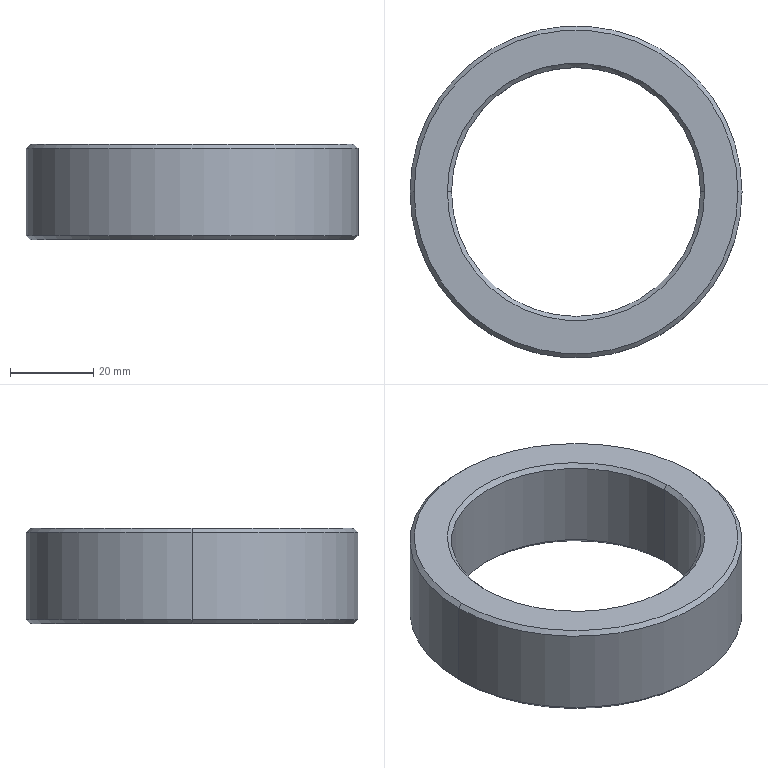Part | SolidWorks | features Chamfer 1, Extrusion 1 | 1 solid | 14 faces | box 80 x 80 x 23 mm | volume 50140 mm3 | cone 8 | cylinder 4 | plane 2 | commonest cylinder face diameters 60 x2 80 x2
STEP:
#1=CARTESIAN_POINT('',(39.,0.,11.5));
#2=VERTEX_POINT('',#1);
#3=CARTESIAN_POINT('',(-39.,0.,11.5));
#4=VERTEX_POINT('',#3);
#5=CARTESIAN_POINT('',(0.,0.,11.5));
#6=DIRECTION('',(0.,0.,1.));
#7=DIRECTION('',(1.,0.,0.));
#8=AXIS2_PLACEMENT_3D('',#5,#6,#7);
#9=CIRCLE('',#8,39.);
#10=EDGE_CURVE('',#2,#4,#9,.T.);
#11=ORIENTED_EDGE('',*,*,#10,.F.);
#12=CARTESIAN_POINT('',(40.,0.,10.5));
#13=VERTEX_POINT('',#12);
#14=CARTESIAN_POINT('',(39.,0.,11.5));
#15=DIRECTION('',(0.7071,0.,-0.7071));
#16=VECTOR('',#15,1000.);
#17=LINE('',#14,#16);
#18=EDGE_CURVE('',#2,#13,#17,.T.);
#19=ORIENTED_EDGE('',*,*,#18,.T.);
#20=CARTESIAN_POINT('',(-40.,0.,10.5));
#21=VERTEX_POINT('',#20);
#22=CARTESIAN_POINT('',(0.,0.,10.5));
#23=DIRECTION('',(0.,0.,-1.));
#24=DIRECTION('',(1.,0.,0.));
#25=AXIS2_PLACEMENT_3D('',#22,#23,#24);
#26=CIRCLE('',#25,40.);
#27=EDGE_CURVE('',#21,#13,#26,.T.);
#28=ORIENTED_EDGE('',*,*,#27,.F.);
#29=CARTESIAN_POINT('',(-39.,0.,11.5));
#30=DIRECTION('',(-0.7071,0.,-0.7071));
#31=VECTOR('',#30,1000.);
#32=LINE('',#29,#31);
#33=EDGE_CURVE('',#4,#21,#32,.T.);
#34=ORIENTED_EDGE('',*,*,#33,.F.);
#35=EDGE_LOOP('',(#11,#19,#28,#34));
#36=FACE_OUTER_BOUND('',#35,.T.);
#37=CARTESIAN_POINT('',(0.,0.,11.5));
#38=DIRECTION('',(0.,0.,-1.));
#39=DIRECTION('',(-1.,0.,0.));
#40=AXIS2_PLACEMENT_3D('',#37,#38,#39);
#41=CONICAL_SURFACE('',#40,39.,0.7854);
#42=ADVANCED_FACE('',(#36),#41,.T.);
#43=CARTESIAN_POINT('',(-30.,0.,10.5));
#44=VERTEX_POINT('',#43);
#45=CARTESIAN_POINT('',(30.,0.,10.5));
#46=VERTEX_POINT('',#45);
#47=CARTESIAN_POINT('',(0.,0.,10.5));
#48=DIRECTION('',(0.,0.,1.));
#49=DIRECTION('',(1.,0.,0.));
#50=AXIS2_PLACEMENT_3D('',#47,#48,#49);
#51=CIRCLE('',#50,30.);
#52=EDGE_CURVE('',#44,#46,#51,.T.);
#53=ORIENTED_EDGE('',*,*,#52,.F.);
#54=CARTESIAN_POINT('',(-31.,0.,11.5));
#55=VERTEX_POINT('',#54);
#56=CARTESIAN_POINT('',(-30.,0.,10.5));
#57=DIRECTION('',(-0.7071,0.,0.7071));
#58=VECTOR('',#57,1000.);
#59=LINE('',#56,#58);
#60=EDGE_CURVE('',#44,#55,#59,.T.);
#61=ORIENTED_EDGE('',*,*,#60,.T.);
#62=CARTESIAN_POINT('',(31.,0.,11.5));
#63=VERTEX_POINT('',#62);
#64=CARTESIAN_POINT('',(0.,0.,11.5));
#65=DIRECTION('',(0.,0.,-1.));
#66=DIRECTION('',(1.,0.,0.));
#67=AXIS2_PLACEMENT_3D('',#64,#65,#66);
#68=CIRCLE('',#67,31.);
#69=EDGE_CURVE('',#63,#55,#68,.T.);
#70=ORIENTED_EDGE('',*,*,#69,.F.);
#71=CARTESIAN_POINT('',(30.,0.,10.5));
#72=DIRECTION('',(0.7071,0.,0.7071));
#73=VECTOR('',#72,1000.);
#74=LINE('',#71,#73);
#75=EDGE_CURVE('',#46,#63,#74,.T.);
#76=ORIENTED_EDGE('',*,*,#75,.F.);
#77=EDGE_LOOP('',(#53,#61,#70,#76));
#78=FACE_OUTER_BOUND('',#77,.T.);
#79=CARTESIAN_POINT('',(0.,0.,10.5));
#80=DIRECTION('',(0.,0.,1.));
#81=DIRECTION('',(1.,0.,0.));
#82=AXIS2_PLACEMENT_3D('',#79,#80,#81);
#83=CONICAL_SURFACE('',#82,30.,0.7854);
#84=ADVANCED_FACE('',(#78),#83,.F.);
#85=CARTESIAN_POINT('',(-39.,0.,-11.5));
#86=VERTEX_POINT('',#85);
#87=CARTESIAN_POINT('',(39.,0.,-11.5));
#88=VERTEX_POINT('',#87);
#89=CARTESIAN_POINT('',(0.,0.,-11.5));
#90=DIRECTION('',(0.,0.,-1.));
#91=DIRECTION('',(1.,0.,0.));
#92=AXIS2_PLACEMENT_3D('',#89,#90,#91);
#93=CIRCLE('',#92,39.);
#94=EDGE_CURVE('',#86,#88,#93,.T.);
#95=ORIENTED_EDGE('',*,*,#94,.F.);
#96=CARTESIAN_POINT('',(-40.,0.,-10.5));
#97=VERTEX_POINT('',#96);
#98=CARTESIAN_POINT('',(-40.,0.,-10.5));
#99=DIRECTION('',(-0.7071,0.,0.7071));
#100=VECTOR('',#99,1000.);
#101=LINE('',#98,#100);
#102=EDGE_CURVE('',#86,#97,#101,.T.);
#103=ORIENTED_EDGE('',*,*,#102,.T.);
#104=CARTESIAN_POINT('',(40.,0.,-10.5));
#105=VERTEX_POINT('',#104);
#106=CARTESIAN_POINT('',(0.,0.,-10.5));
#107=DIRECTION('',(0.,0.,1.));
#108=DIRECTION('',(1.,0.,0.));
#109=AXIS2_PLACEMENT_3D('',#106,#107,#108);
#110=CIRCLE('',#109,40.);
#111=EDGE_CURVE('',#105,#97,#110,.T.);
#112=ORIENTED_EDGE('',*,*,#111,.F.);
#113=CARTESIAN_POINT('',(40.,0.,-10.5));
#114=DIRECTION('',(0.7071,0.,0.7071));
#115=VECTOR('',#114,1000.);
#116=LINE('',#113,#115);
#117=EDGE_CURVE('',#88,#105,#116,.T.);
#118=ORIENTED_EDGE('',*,*,#117,.F.);
#119=EDGE_LOOP('',(#95,#103,#112,#118));
#120=FACE_OUTER_BOUND('',#119,.T.);
#121=CARTESIAN_POINT('',(0.,0.,-10.5));
#122=DIRECTION('',(0.,0.,1.));
#123=DIRECTION('',(1.,0.,0.));
#124=AXIS2_PLACEMENT_3D('',#121,#122,#123);
#125=CONICAL_SURFACE('',#124,40.,0.7854);
#126=ADVANCED_FACE('',(#120),#125,.T.);
#127=CARTESIAN_POINT('',(30.,0.,-10.5));
#128=VERTEX_POINT('',#127);
#129=CARTESIAN_POINT('',(-30.,0.,-10.5));
#130=VERTEX_POINT('',#129);
#131=CARTESIAN_POINT('',(0.,0.,-10.5));
#132=DIRECTION('',(0.,0.,-1.));
#133=DIRECTION('',(1.,0.,0.));
#134=AXIS2_PLACEMENT_3D('',#131,#132,#133);
#135=CIRCLE('',#134,30.);
#136=EDGE_CURVE('',#128,#130,#135,.T.);
#137=ORIENTED_EDGE('',*,*,#136,.F.);
#138=CARTESIAN_POINT('',(31.,0.,-11.5));
#139=VERTEX_POINT('',#138);
#140=CARTESIAN_POINT('',(31.,0.,-11.5));
#141=DIRECTION('',(0.7071,0.,-0.7071));
#142=VECTOR('',#141,1000.);
#143=LINE('',#140,#142);
#144=EDGE_CURVE('',#128,#139,#143,.T.);
#145=ORIENTED_EDGE('',*,*,#144,.T.);
#146=CARTESIAN_POINT('',(-31.,0.,-11.5));
#147=VERTEX_POINT('',#146);
#148=CARTESIAN_POINT('',(0.,0.,-11.5));
#149=DIRECTION('',(0.,0.,1.));
#150=DIRECTION('',(1.,0.,0.));
#151=AXIS2_PLACEMENT_3D('',#148,#149,#150);
#152=CIRCLE('',#151,31.);
#153=EDGE_CURVE('',#147,#139,#152,.T.);
#154=ORIENTED_EDGE('',*,*,#153,.F.);
#155=CARTESIAN_POINT('',(-31.,0.,-11.5));
#156=DIRECTION('',(-0.7071,0.,-0.7071));
#157=VECTOR('',#156,1000.);
#158=LINE('',#155,#157);
#159=EDGE_CURVE('',#130,#147,#158,.T.);
#160=ORIENTED_EDGE('',*,*,#159,.F.);
#161=EDGE_LOOP('',(#137,#145,#154,#160));
#162=FACE_OUTER_BOUND('',#161,.T.);
#163=CARTESIAN_POINT('',(0.,0.,-11.5));
#164=DIRECTION('',(0.,0.,-1.));
#165=DIRECTION('',(-1.,0.,0.));
#166=AXIS2_PLACEMENT_3D('',#163,#164,#165);
#167=CONICAL_SURFACE('',#166,31.,0.7854);
#168=ADVANCED_FACE('',(#162),#167,.F.);
#169=ORIENTED_EDGE('',*,*,#52,.T.);
#170=CARTESIAN_POINT('',(30.,0.,11.5));
#171=DIRECTION('',(0.,0.,-1.));
#172=VECTOR('',#171,1000.);
#173=LINE('',#170,#172);
#174=EDGE_CURVE('',#46,#128,#173,.T.);
#175=ORIENTED_EDGE('',*,*,#174,.T.);
#176=ORIENTED_EDGE('',*,*,#136,.T.);
#177=CARTESIAN_POINT('',(-30.,0.,11.5));
#178=DIRECTION('',(0.,0.,-1.));
#179=VECTOR('',#178,1000.);
#180=LINE('',#177,#179);
#181=EDGE_CURVE('',#44,#130,#180,.T.);
#182=ORIENTED_EDGE('',*,*,#181,.F.);
#183=EDGE_LOOP('',(#169,#175,#176,#182));
#184=FACE_OUTER_BOUND('',#183,.T.);
#185=CARTESIAN_POINT('',(0.,0.,11.5));
#186=DIRECTION('',(0.,0.,-1.));
#187=DIRECTION('',(-1.,0.,0.));
#188=AXIS2_PLACEMENT_3D('',#185,#186,#187);
#189=CYLINDRICAL_SURFACE('',#188,30.);
#190=ADVANCED_FACE('',(#184),#189,.F.);
#191=ORIENTED_EDGE('',*,*,#27,.T.);
#192=CARTESIAN_POINT('',(40.,0.,11.5));
#193=DIRECTION('',(0.,0.,-1.));
#194=VECTOR('',#193,1000.);
#195=LINE('',#192,#194);
#196=EDGE_CURVE('',#13,#105,#195,.T.);
#197=ORIENTED_EDGE('',*,*,#196,.T.);
#198=ORIENTED_EDGE('',*,*,#111,.T.);
#199=CARTESIAN_POINT('',(-40.,0.,11.5));
#200=DIRECTION('',(0.,0.,-1.));
#201=VECTOR('',#200,1000.);
#202=LINE('',#199,#201);
#203=EDGE_CURVE('',#21,#97,#202,.T.);
#204=ORIENTED_EDGE('',*,*,#203,.F.);
#205=EDGE_LOOP('',(#191,#197,#198,#204));
#206=FACE_OUTER_BOUND('',#205,.T.);
#207=CARTESIAN_POINT('',(0.,0.,11.5));
#208=DIRECTION('',(0.,0.,-1.));
#209=DIRECTION('',(-1.,0.,0.));
#210=AXIS2_PLACEMENT_3D('',#207,#208,#209);
#211=CYLINDRICAL_SURFACE('',#210,40.);
#212=ADVANCED_FACE('',(#206),#211,.T.);
#213=ORIENTED_EDGE('',*,*,#69,.T.);
#214=CARTESIAN_POINT('',(0.,0.,11.5));
#215=DIRECTION('',(0.,0.,-1.));
#216=DIRECTION('',(1.,0.,0.));
#217=AXIS2_PLACEMENT_3D('',#214,#215,#216);
#218=CIRCLE('',#217,31.);
#219=EDGE_CURVE('',#55,#63,#218,.T.);
#220=ORIENTED_EDGE('',*,*,#219,.T.);
#221=EDGE_LOOP('',(#213,#220));
#222=FACE_BOUND('',#221,.T.);
#223=CARTESIAN_POINT('',(0.,0.,11.5));
#224=DIRECTION('',(0.,0.,1.));
#225=DIRECTION('',(1.,0.,0.));
#226=AXIS2_PLACEMENT_3D('',#223,#224,#225);
#227=CIRCLE('',#226,39.);
#228=EDGE_CURVE('',#4,#2,#227,.T.);
#229=ORIENTED_EDGE('',*,*,#228,.T.);
#230=ORIENTED_EDGE('',*,*,#10,.T.);
#231=EDGE_LOOP('',(#229,#230));
#232=FACE_OUTER_BOUND('',#231,.T.);
#233=CARTESIAN_POINT('',(0.,0.,11.5));
#234=DIRECTION('',(0.,0.,1.));
#235=DIRECTION('',(1.,0.,0.));
#236=AXIS2_PLACEMENT_3D('',#233,#234,#235);
#237=PLANE('',#236);
#238=ADVANCED_FACE('',(#222,#232),#237,.T.);
#239=ORIENTED_EDGE('',*,*,#153,.T.);
#240=CARTESIAN_POINT('',(0.,0.,-11.5));
#241=DIRECTION('',(0.,0.,1.));
#242=DIRECTION('',(1.,0.,0.));
#243=AXIS2_PLACEMENT_3D('',#240,#241,#242);
#244=CIRCLE('',#243,31.);
#245=EDGE_CURVE('',#139,#147,#244,.T.);
#246=ORIENTED_EDGE('',*,*,#245,.T.);
#247=EDGE_LOOP('',(#239,#246));
#248=FACE_BOUND('',#247,.T.);
#249=CARTESIAN_POINT('',(0.,0.,-11.5));
#250=DIRECTION('',(0.,0.,-1.));
#251=DIRECTION('',(1.,0.,0.));
#252=AXIS2_PLACEMENT_3D('',#249,#250,#251);
#253=CIRCLE('',#252,39.);
#254=EDGE_CURVE('',#88,#86,#253,.T.);
#255=ORIENTED_EDGE('',*,*,#254,.T.);
#256=ORIENTED_EDGE('',*,*,#94,.T.);
#257=EDGE_LOOP('',(#255,#256));
#258=FACE_OUTER_BOUND('',#257,.T.);
#259=CARTESIAN_POINT('',(0.,0.,-11.5));
#260=DIRECTION('',(0.,0.,1.));
#261=DIRECTION('',(1.,0.,0.));
#262=AXIS2_PLACEMENT_3D('',#259,#260,#261);
#263=PLANE('',#262);
#264=ADVANCED_FACE('',(#248,#258),#263,.F.);
#265=ORIENTED_EDGE('',*,*,#196,.F.);
#266=CARTESIAN_POINT('',(0.,0.,10.5));
#267=DIRECTION('',(0.,0.,-1.));
#268=DIRECTION('',(1.,0.,0.));
#269=AXIS2_PLACEMENT_3D('',#266,#267,#268);
#270=CIRCLE('',#269,40.);
#271=EDGE_CURVE('',#13,#21,#270,.T.);
#272=ORIENTED_EDGE('',*,*,#271,.T.);
#273=ORIENTED_EDGE('',*,*,#203,.T.);
#274=CARTESIAN_POINT('',(0.,0.,-10.5));
#275=DIRECTION('',(0.,0.,1.));
#276=DIRECTION('',(1.,0.,0.));
#277=AXIS2_PLACEMENT_3D('',#274,#275,#276);
#278=CIRCLE('',#277,40.);
#279=EDGE_CURVE('',#97,#105,#278,.T.);
#280=ORIENTED_EDGE('',*,*,#279,.T.);
#281=EDGE_LOOP('',(#265,#272,#273,#280));
#282=FACE_OUTER_BOUND('',#281,.T.);
#283=CARTESIAN_POINT('',(0.,0.,11.5));
#284=DIRECTION('',(0.,0.,-1.));
#285=DIRECTION('',(-1.,0.,0.));
#286=AXIS2_PLACEMENT_3D('',#283,#284,#285);
#287=CYLINDRICAL_SURFACE('',#286,40.);
#288=ADVANCED_FACE('',(#282),#287,.T.);
#289=ORIENTED_EDGE('',*,*,#174,.F.);
#290=CARTESIAN_POINT('',(0.,0.,10.5));
#291=DIRECTION('',(0.,0.,1.));
#292=DIRECTION('',(1.,0.,0.));
#293=AXIS2_PLACEMENT_3D('',#290,#291,#292);
#294=CIRCLE('',#293,30.);
#295=EDGE_CURVE('',#46,#44,#294,.T.);
#296=ORIENTED_EDGE('',*,*,#295,.T.);
#297=ORIENTED_EDGE('',*,*,#181,.T.);
#298=CARTESIAN_POINT('',(0.,0.,-10.5));
#299=DIRECTION('',(0.,0.,-1.));
#300=DIRECTION('',(1.,0.,0.));
#301=AXIS2_PLACEMENT_3D('',#298,#299,#300);
#302=CIRCLE('',#301,30.);
#303=EDGE_CURVE('',#130,#128,#302,.T.);
#304=ORIENTED_EDGE('',*,*,#303,.T.);
#305=EDGE_LOOP('',(#289,#296,#297,#304));
#306=FACE_OUTER_BOUND('',#305,.T.);
#307=CARTESIAN_POINT('',(0.,0.,11.5));
#308=DIRECTION('',(0.,0.,-1.));
#309=DIRECTION('',(-1.,0.,0.));
#310=AXIS2_PLACEMENT_3D('',#307,#308,#309);
#311=CYLINDRICAL_SURFACE('',#310,30.);
#312=ADVANCED_FACE('',(#306),#311,.F.);
#313=ORIENTED_EDGE('',*,*,#144,.F.);
#314=ORIENTED_EDGE('',*,*,#303,.F.);
#315=ORIENTED_EDGE('',*,*,#159,.T.);
#316=ORIENTED_EDGE('',*,*,#245,.F.);
#317=EDGE_LOOP('',(#313,#314,#315,#316));
#318=FACE_OUTER_BOUND('',#317,.T.);
#319=CARTESIAN_POINT('',(0.,0.,-11.5));
#320=DIRECTION('',(0.,0.,-1.));
#321=DIRECTION('',(-1.,0.,0.));
#322=AXIS2_PLACEMENT_3D('',#319,#320,#321);
#323=CONICAL_SURFACE('',#322,31.,0.7854);
#324=ADVANCED_FACE('',(#318),#323,.F.);
#325=ORIENTED_EDGE('',*,*,#102,.F.);
#326=ORIENTED_EDGE('',*,*,#254,.F.);
#327=ORIENTED_EDGE('',*,*,#117,.T.);
#328=ORIENTED_EDGE('',*,*,#279,.F.);
#329=EDGE_LOOP('',(#325,#326,#327,#328));
#330=FACE_OUTER_BOUND('',#329,.T.);
#331=CARTESIAN_POINT('',(0.,0.,-10.5));
#332=DIRECTION('',(0.,0.,1.));
#333=DIRECTION('',(1.,0.,0.));
#334=AXIS2_PLACEMENT_3D('',#331,#332,#333);
#335=CONICAL_SURFACE('',#334,40.,0.7854);
#336=ADVANCED_FACE('',(#330),#335,.T.);
#337=ORIENTED_EDGE('',*,*,#60,.F.);
#338=ORIENTED_EDGE('',*,*,#295,.F.);
#339=ORIENTED_EDGE('',*,*,#75,.T.);
#340=ORIENTED_EDGE('',*,*,#219,.F.);
#341=EDGE_LOOP('',(#337,#338,#339,#340));
#342=FACE_OUTER_BOUND('',#341,.T.);
#343=CARTESIAN_POINT('',(0.,0.,10.5));
#344=DIRECTION('',(0.,0.,1.));
#345=DIRECTION('',(1.,0.,0.));
#346=AXIS2_PLACEMENT_3D('',#343,#344,#345);
#347=CONICAL_SURFACE('',#346,30.,0.7854);
#348=ADVANCED_FACE('',(#342),#347,.F.);
#349=ORIENTED_EDGE('',*,*,#18,.F.);
#350=ORIENTED_EDGE('',*,*,#228,.F.);
#351=ORIENTED_EDGE('',*,*,#33,.T.);
#352=ORIENTED_EDGE('',*,*,#271,.F.);
#353=EDGE_LOOP('',(#349,#350,#351,#352));
#354=FACE_OUTER_BOUND('',#353,.T.);
#355=CARTESIAN_POINT('',(0.,0.,11.5));
#356=DIRECTION('',(0.,0.,-1.));
#357=DIRECTION('',(-1.,0.,0.));
#358=AXIS2_PLACEMENT_3D('',#355,#356,#357);
#359=CONICAL_SURFACE('',#358,39.,0.7854);
#360=ADVANCED_FACE('',(#354),#359,.T.);
#361=CLOSED_SHELL('',(#42,#84,#126,#168,#190,#212,#238,#264,#288,#312,#324,#336,#348,#360));
#362=MANIFOLD_SOLID_BREP('',#361);
#363=CARTESIAN_POINT('',(0.,0.,0.));
#364=DIRECTION('',(0.,0.,1.));
#365=DIRECTION('',(1.,0.,0.));
#366=AXIS2_PLACEMENT_3D('',#363,#364,#365);
#367=(LENGTH_UNIT()NAMED_UNIT(*)SI_UNIT(.MILLI.,.METRE.));
#368=UNCERTAINTY_MEASURE_WITH_UNIT(LENGTH_MEASURE(0.00001),#367,'','');
#369=(NAMED_UNIT(*)PLANE_ANGLE_UNIT()SI_UNIT($,.RADIAN.));
#370=(NAMED_UNIT(*)SI_UNIT($,.STERADIAN.)SOLID_ANGLE_UNIT());
#371=(GEOMETRIC_REPRESENTATION_CONTEXT(3)GLOBAL_UNCERTAINTY_ASSIGNED_CONTEXT((#368))GLOBAL_UNIT_ASSIGNED_CONTEXT((#367,#369,#370))REPRESENTATION_CONTEXT('',''));
#372=ADVANCED_BREP_SHAPE_REPRESENTATION('',(#362,#366),#371);